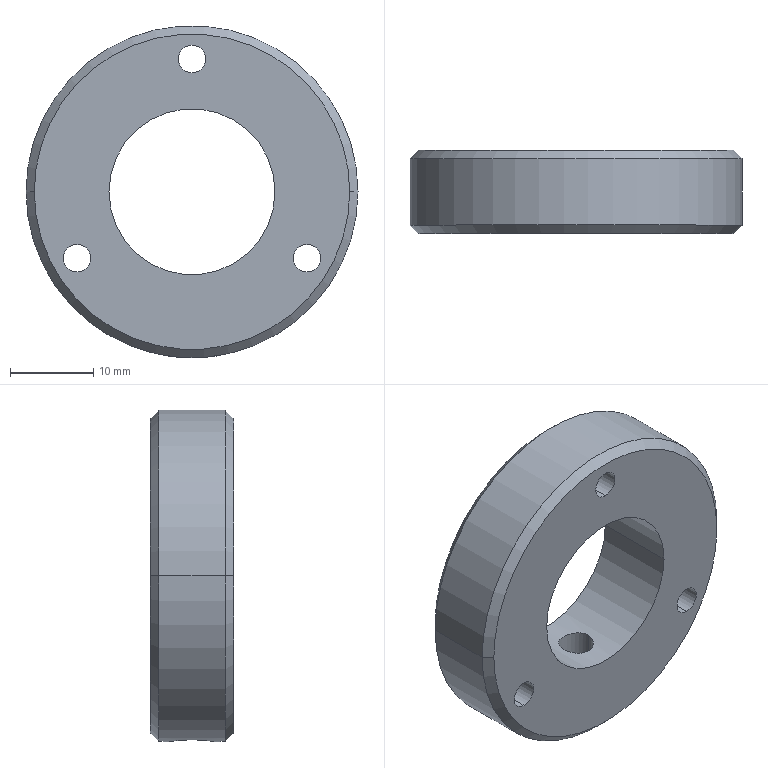Part | STEP file | QA-FC11 | 1 solid | 20 faces | box 40 x 10 x 40 mm | volume 8899 mm3 | cylinder 12 | cone 4 | spline 2 | plane 2 | commonest cylinder face diameters 3.3 x6 4.2 x2 20 x2 40 x2